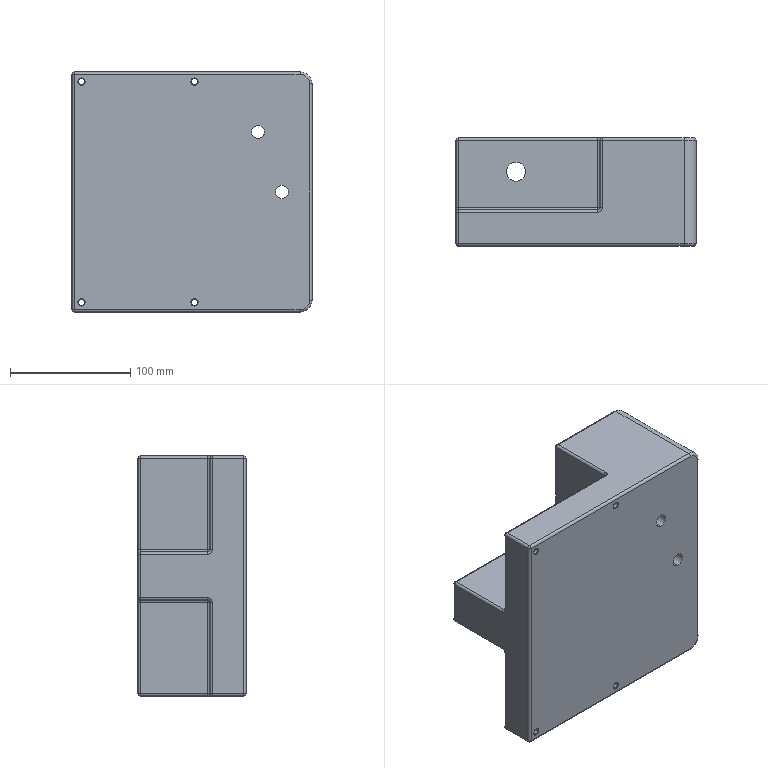Part | SolidWorks | features ICE 8, Fillet 2, MoveFace 2, Extrusion 1, HoleWzd 1 | 1 solid | 97 faces | box 200 x 90 x 200 mm | volume 2336478 mm3 | cylinder 54 | plane 15 | torus 10 | sphere 10 | cone 8 | commonest cylinder face diameters 4 x28 5 x8 11 x8 20 x4 16 x2 31 x2